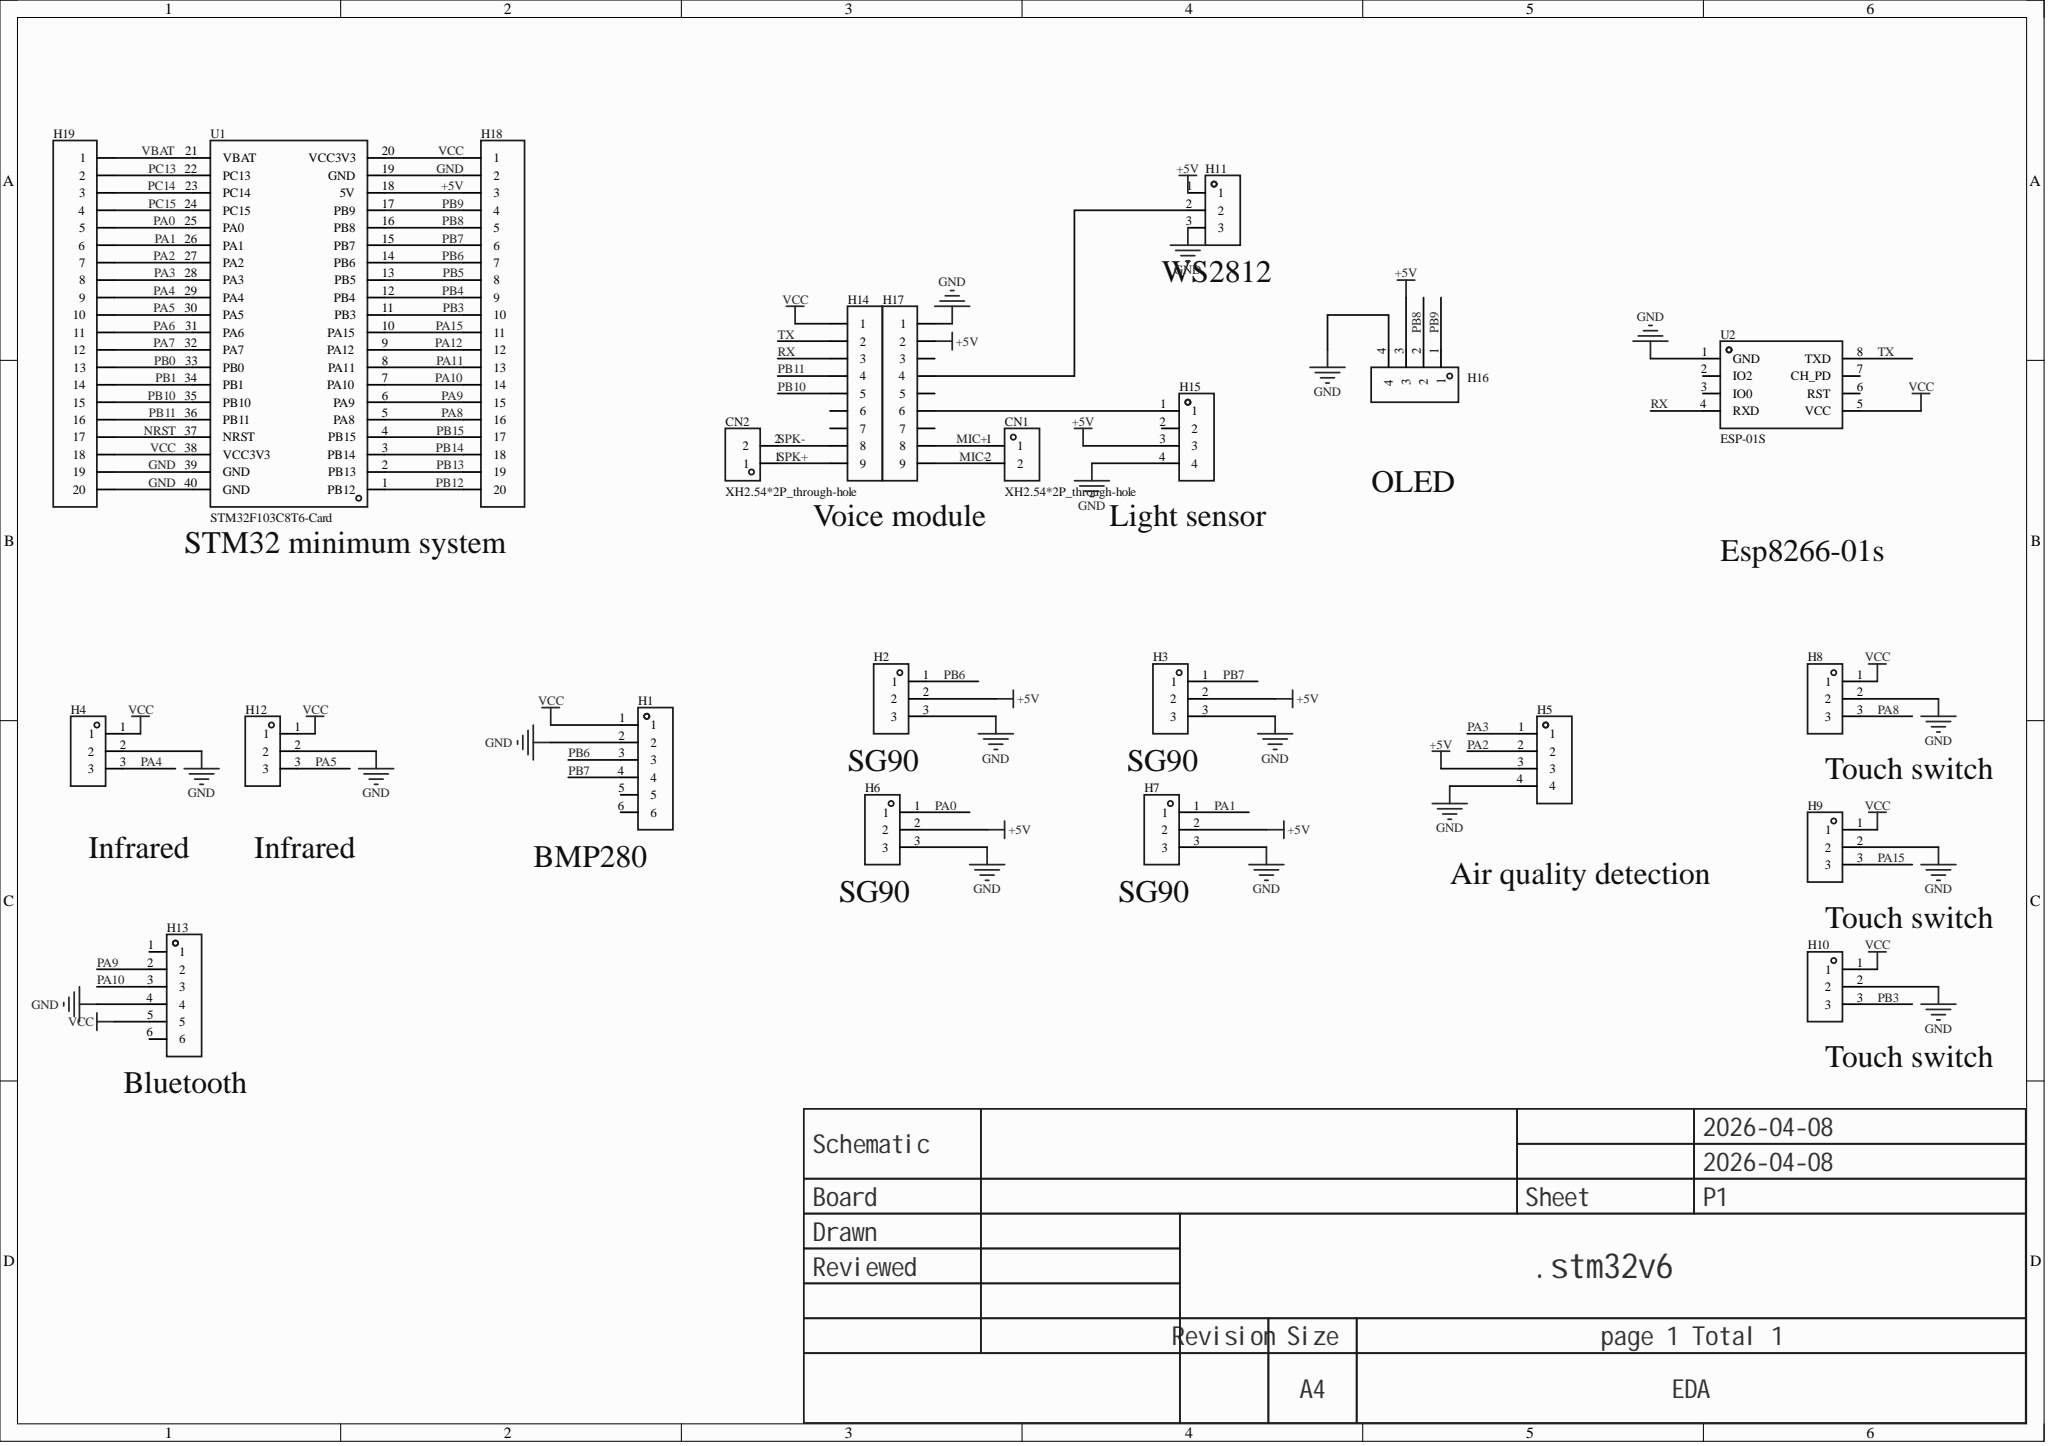Circuit board | Altium Designer | 23 parts | 45 nets
Bill of materials:
Comment,Description,Designator,Footprint,LibRef,Quantity
"XH2.54*2P_through-hole","","CN1, CN2","CONN-TH_2P-P2.50-XH2.54-2P","XH2.54*2P_直插","2"
"","","H1, H13","HDR-TH_6P-P2.54-V-F","HDR-F_2.54_1x6P","2"
"","","H2, H3, H4, H6, H7, H8, H9, H10, H11, H12","HDR-TH_3P-P2.54-V-F","HDR-F_2.54_1x3P","10"
"","","H5, H15, H16","HDR-TH_4P-P2.54-V-F","HDR-F_2.54_1x4P","3"
"","","H14, H17","HDR-TH_9P-P2.54-V-F-1","HDR-F_2.54_1x9P","2"
"","","H18, H19","HDR-TH_20P-P2.54-V-F","HDR-F_2.54_1x20P","2"
"STM32F103C8T6-Card","","U1","CONN-TH_L53.3-W22.9_STM32F103C8T6-CARD","STM32F103C8T6-Card","1"
"ESP-01S","","U2","WIFIM-TH_ESP-01S","ESP-01S_C111009","1"
Netlist (Protel format):
[
CN1
CONN-TH_2P-P2.50-XH2.54-2P
XH2.54*2P_through-hole



]
[
CN2
CONN-TH_2P-P2.50-XH2.54-2P
XH2.54*2P_through-hole



]
[
H1
HDR-TH_6P-P2.54-V-F




]
[
H2
HDR-TH_3P-P2.54-V-F




]
[
H3
HDR-TH_3P-P2.54-V-F




]
[
H4
HDR-TH_3P-P2.54-V-F




]
[
H5
HDR-TH_4P-P2.54-V-F




]
[
H6
HDR-TH_3P-P2.54-V-F




]
[
H7
HDR-TH_3P-P2.54-V-F




]
[
H8
HDR-TH_3P-P2.54-V-F




]
[
H9
HDR-TH_3P-P2.54-V-F




]
[
H10
HDR-TH_3P-P2.54-V-F




]
[
H11
HDR-TH_3P-P2.54-V-F




]
[
H12
HDR-TH_3P-P2.54-V-F




]
[
H13
HDR-TH_6P-P2.54-V-F




]
[
H14
HDR-TH_9P-P2.54-V-F-1




]
[
H15
HDR-TH_4P-P2.54-V-F




]
[
H16
HDR-TH_4P-P2.54-V-F




]
[
H17
HDR-TH_9P-P2.54-V-F-1




]
[
H18
HDR-TH_20P-P2.54-V-F




]
[
H19
HDR-TH_20P-P2.54-V-F




]
[
U1
CONN-TH_L53.3-W22.9_STM32F103C8T6-CARD
STM32F103C8T6-Card



]
[
U2
WIFIM-TH_ESP-01S
ESP-01S



]
(
VCC
H1-1
H4-1
H8-1
H9-1
H10-1
H12-1
H13-5
H14-1
H18-1
H19-18
U1-20
U1-38
U2-5
)
(
VBAT
H19-1
U1-21
)
(
TX
H14-2
U2-8
)
(
SPK-
CN2-2
H14-8
)
(
SPK+
CN2-1
H14-9
)
(
RX
H14-3
U2-4
)
(
PC15
H19-4
U1-24
)
(
PC14
H19-3
U1-23
)
(
PC13
H19-2
U1-22
)
(
PB15
H18-17
U1-4
)
(
PB14
H18-18
U1-3
)
(
PB13
H18-19
U1-2
)
(
PB12
H18-20
U1-1
)
(
PB11
H14-4
H19-16
U1-36
)
(
PB10
H14-5
H19-15
U1-35
)
(
PB9
H16-1
H18-4
U1-17
)
(
PB8
H16-2
H18-5
U1-16
)
(
PB7
H1-4
H3-1
H18-6
U1-15
)
(
PB6
H1-3
H2-1
H18-7
U1-14
)
(
PB5
H18-8
U1-13
)
(
PB4
H18-9
U1-12
)
(
PB3
H10-3
H18-10
U1-11
)
(
PB1
H19-14
U1-34
)
(
PB0
H19-13
U1-33
)
(
PA15
H9-3
H18-11
U1-10
)
(
PA12
H18-12
U1-9
)
(
PA11
H18-13
U1-8
)
(
PA10
H13-3
H18-14
U1-7
)
(
PA9
H13-2
H18-15
U1-6
)
(
PA8
H8-3
H18-16
U1-5
)
(
PA7
H19-12
U1-32
)
(
PA6
H19-11
U1-31
)
(
PA5
H12-3
H19-10
U1-30
)
(
PA4
H4-3
H19-9
U1-29
)
(
PA3
H5-1
H19-8
U1-28
)
(
PA2
H5-2
H19-7
U1-27
)
(
PA1
H7-1
H19-6
U1-26
)
(
PA0
H6-1
H19-5
U1-25
)
(
NRST
H19-17
U1-37
)
(
NetH15_1
H15-1
H17-6
)
(
NetH11_2
H11-2
H17-4
)
(
MIC-
CN1-2
H17-9
)
(
MIC+
CN1-1
H17-8
)
(
GND
H1-2
H2-3
H3-3
H4-2
H5-4
H6-3
H7-3
H8-2
H9-2
H10-2
H11-3
H12-2
H13-4
H15-4
H16-4
H17-1
H18-2
H19-19
H19-20
U1-19
U1-39
U1-40
U2-1
)
(
+5V
H2-2
H3-2
H5-3
H6-2
H7-2
H11-1
H15-3
H16-3
H17-2
H18-3
U1-18
)